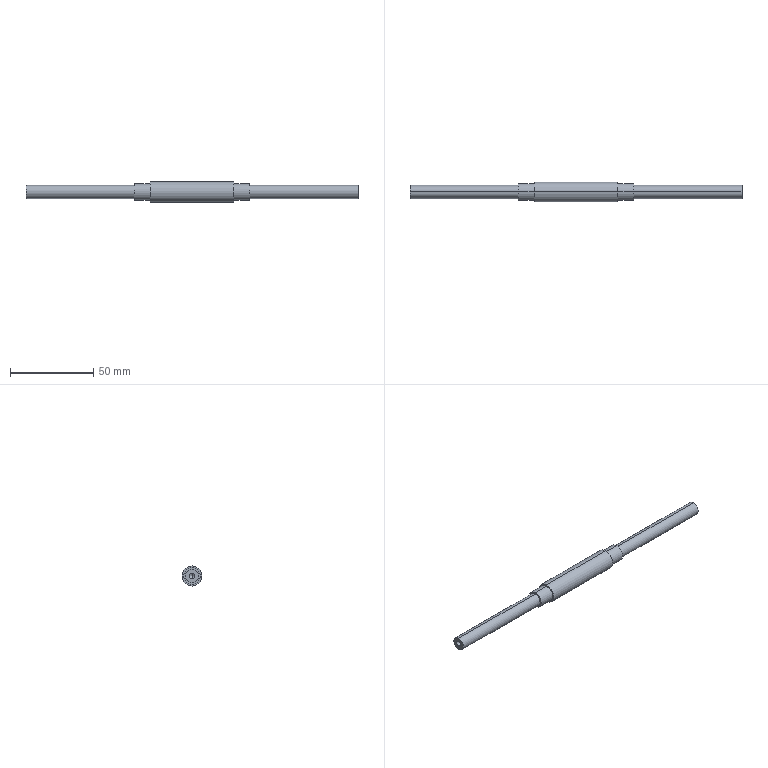Part | STEP file | MT-COMBO-119-S036 | 1 solid | 24 faces | box 199 x 12 x 12 mm | volume 13503 mm3 | cylinder 14 | plane 6 | cone 4 | commonest cylinder face diameters 3.3 x4 8 x4 10 x4 12 x2
STEP:
#1=CARTESIAN_POINT('',(89.4,0.,1.65));
#2=VERTEX_POINT('',#1);
#3=CARTESIAN_POINT('',(89.4,0.,-1.65));
#4=VERTEX_POINT('',#3);
#5=CARTESIAN_POINT('',(89.4,0.,0.));
#6=DIRECTION('',(-1.,0.,0.));
#7=DIRECTION('',(0.,0.,1.));
#8=AXIS2_PLACEMENT_3D('',#5,#6,#7);
#9=CIRCLE('',#8,1.65);
#10=EDGE_CURVE('',#2,#4,#9,.T.);
#11=ORIENTED_EDGE('',*,*,#10,.T.);
#12=CARTESIAN_POINT('',(99.5,0.,-1.65));
#13=VERTEX_POINT('',#12);
#14=CARTESIAN_POINT('',(99.5,0.,-1.65));
#15=DIRECTION('',(1.,0.,0.));
#16=VECTOR('',#15,1000.);
#17=LINE('',#14,#16);
#18=EDGE_CURVE('',#4,#13,#17,.T.);
#19=ORIENTED_EDGE('',*,*,#18,.T.);
#20=CARTESIAN_POINT('',(99.5,0.,1.65));
#21=VERTEX_POINT('',#20);
#22=CARTESIAN_POINT('',(99.5,0.,0.));
#23=DIRECTION('',(-1.,0.,0.));
#24=DIRECTION('',(0.,0.,1.));
#25=AXIS2_PLACEMENT_3D('',#22,#23,#24);
#26=CIRCLE('',#25,1.65);
#27=EDGE_CURVE('',#21,#13,#26,.T.);
#28=ORIENTED_EDGE('',*,*,#27,.F.);
#29=CARTESIAN_POINT('',(99.5,0.,1.65));
#30=DIRECTION('',(1.,0.,0.));
#31=VECTOR('',#30,1000.);
#32=LINE('',#29,#31);
#33=EDGE_CURVE('',#2,#21,#32,.T.);
#34=ORIENTED_EDGE('',*,*,#33,.F.);
#35=EDGE_LOOP('',(#11,#19,#28,#34));
#36=FACE_OUTER_BOUND('',#35,.T.);
#37=CARTESIAN_POINT('',(99.5,0.,0.));
#38=DIRECTION('',(1.,0.,0.));
#39=DIRECTION('',(0.,0.,1.));
#40=AXIS2_PLACEMENT_3D('',#37,#38,#39);
#41=CYLINDRICAL_SURFACE('',#40,1.65);
#42=ADVANCED_FACE('',(#36),#41,.F.);
#43=CARTESIAN_POINT('',(88.409,0.,0.));
#44=VERTEX_POINT('',#43);
#45=CARTESIAN_POINT('',(89.4,0.,1.65));
#46=DIRECTION('',(0.515,0.,0.8572));
#47=VECTOR('',#46,1000.);
#48=LINE('',#45,#47);
#49=EDGE_CURVE('',#44,#2,#48,.T.);
#50=ORIENTED_EDGE('',*,*,#49,.F.);
#51=CARTESIAN_POINT('',(89.4,0.,-1.65));
#52=DIRECTION('',(0.515,0.,-0.8572));
#53=VECTOR('',#52,1000.);
#54=LINE('',#51,#53);
#55=EDGE_CURVE('',#44,#4,#54,.T.);
#56=ORIENTED_EDGE('',*,*,#55,.T.);
#57=ORIENTED_EDGE('',*,*,#10,.F.);
#58=EDGE_LOOP('',(#50,#56,#57));
#59=FACE_OUTER_BOUND('',#58,.T.);
#60=CARTESIAN_POINT('',(89.4,0.,0.));
#61=DIRECTION('',(1.,0.,0.));
#62=DIRECTION('',(0.,0.,1.));
#63=AXIS2_PLACEMENT_3D('',#60,#61,#62);
#64=CONICAL_SURFACE('',#63,1.65,1.03);
#65=ADVANCED_FACE('',(#59),#64,.F.);
#66=CARTESIAN_POINT('',(-89.4,0.,-1.65));
#67=VERTEX_POINT('',#66);
#68=CARTESIAN_POINT('',(-89.4,0.,1.65));
#69=VERTEX_POINT('',#68);
#70=CARTESIAN_POINT('',(-89.4,0.,0.));
#71=DIRECTION('',(1.,0.,0.));
#72=DIRECTION('',(0.,0.,-1.));
#73=AXIS2_PLACEMENT_3D('',#70,#71,#72);
#74=CIRCLE('',#73,1.65);
#75=EDGE_CURVE('',#67,#69,#74,.T.);
#76=ORIENTED_EDGE('',*,*,#75,.T.);
#77=CARTESIAN_POINT('',(-99.5,0.,1.65));
#78=VERTEX_POINT('',#77);
#79=CARTESIAN_POINT('',(-99.5,0.,1.65));
#80=DIRECTION('',(-1.,0.,0.));
#81=VECTOR('',#80,1000.);
#82=LINE('',#79,#81);
#83=EDGE_CURVE('',#69,#78,#82,.T.);
#84=ORIENTED_EDGE('',*,*,#83,.T.);
#85=CARTESIAN_POINT('',(-99.5,0.,-1.65));
#86=VERTEX_POINT('',#85);
#87=CARTESIAN_POINT('',(-99.5,0.,0.));
#88=DIRECTION('',(1.,0.,0.));
#89=DIRECTION('',(0.,0.,-1.));
#90=AXIS2_PLACEMENT_3D('',#87,#88,#89);
#91=CIRCLE('',#90,1.65);
#92=EDGE_CURVE('',#86,#78,#91,.T.);
#93=ORIENTED_EDGE('',*,*,#92,.F.);
#94=CARTESIAN_POINT('',(-99.5,0.,-1.65));
#95=DIRECTION('',(-1.,0.,0.));
#96=VECTOR('',#95,1000.);
#97=LINE('',#94,#96);
#98=EDGE_CURVE('',#67,#86,#97,.T.);
#99=ORIENTED_EDGE('',*,*,#98,.F.);
#100=EDGE_LOOP('',(#76,#84,#93,#99));
#101=FACE_OUTER_BOUND('',#100,.T.);
#102=CARTESIAN_POINT('',(-99.5,0.,0.));
#103=DIRECTION('',(-1.,0.,0.));
#104=DIRECTION('',(0.,0.,-1.));
#105=AXIS2_PLACEMENT_3D('',#102,#103,#104);
#106=CYLINDRICAL_SURFACE('',#105,1.65);
#107=ADVANCED_FACE('',(#101),#106,.F.);
#108=CARTESIAN_POINT('',(-88.409,0.,0.));
#109=VERTEX_POINT('',#108);
#110=CARTESIAN_POINT('',(-89.4,0.,-1.65));
#111=DIRECTION('',(-0.515,0.,-0.8572));
#112=VECTOR('',#111,1000.);
#113=LINE('',#110,#112);
#114=EDGE_CURVE('',#109,#67,#113,.T.);
#115=ORIENTED_EDGE('',*,*,#114,.F.);
#116=CARTESIAN_POINT('',(-89.4,0.,1.65));
#117=DIRECTION('',(-0.515,0.,0.8572));
#118=VECTOR('',#117,1000.);
#119=LINE('',#116,#118);
#120=EDGE_CURVE('',#109,#69,#119,.T.);
#121=ORIENTED_EDGE('',*,*,#120,.T.);
#122=ORIENTED_EDGE('',*,*,#75,.F.);
#123=EDGE_LOOP('',(#115,#121,#122));
#124=FACE_OUTER_BOUND('',#123,.T.);
#125=CARTESIAN_POINT('',(-89.4,0.,0.));
#126=DIRECTION('',(-1.,0.,0.));
#127=DIRECTION('',(0.,0.,-1.));
#128=AXIS2_PLACEMENT_3D('',#125,#126,#127);
#129=CONICAL_SURFACE('',#128,1.65,1.03);
#130=ADVANCED_FACE('',(#124),#129,.F.);
#131=CARTESIAN_POINT('',(-34.5,0.,4.));
#132=VERTEX_POINT('',#131);
#133=CARTESIAN_POINT('',(-34.5,0.,-4.));
#134=VERTEX_POINT('',#133);
#135=CARTESIAN_POINT('',(-34.5,0.,0.));
#136=DIRECTION('',(1.,0.,0.));
#137=DIRECTION('',(0.,0.,-1.));
#138=AXIS2_PLACEMENT_3D('',#135,#136,#137);
#139=CIRCLE('',#138,4.);
#140=EDGE_CURVE('',#132,#134,#139,.T.);
#141=ORIENTED_EDGE('',*,*,#140,.F.);
#142=CARTESIAN_POINT('',(-99.5,0.,4.));
#143=VERTEX_POINT('',#142);
#144=CARTESIAN_POINT('',(-99.5,0.,4.));
#145=DIRECTION('',(-1.,0.,0.));
#146=VECTOR('',#145,1000.);
#147=LINE('',#144,#146);
#148=EDGE_CURVE('',#132,#143,#147,.T.);
#149=ORIENTED_EDGE('',*,*,#148,.T.);
#150=CARTESIAN_POINT('',(-99.5,0.,-4.));
#151=VERTEX_POINT('',#150);
#152=CARTESIAN_POINT('',(-99.5,0.,0.));
#153=DIRECTION('',(1.,0.,0.));
#154=DIRECTION('',(0.,0.,-1.));
#155=AXIS2_PLACEMENT_3D('',#152,#153,#154);
#156=CIRCLE('',#155,4.);
#157=EDGE_CURVE('',#143,#151,#156,.T.);
#158=ORIENTED_EDGE('',*,*,#157,.T.);
#159=CARTESIAN_POINT('',(-99.5,0.,-4.));
#160=DIRECTION('',(-1.,0.,0.));
#161=VECTOR('',#160,1000.);
#162=LINE('',#159,#161);
#163=EDGE_CURVE('',#134,#151,#162,.T.);
#164=ORIENTED_EDGE('',*,*,#163,.F.);
#165=EDGE_LOOP('',(#141,#149,#158,#164));
#166=FACE_OUTER_BOUND('',#165,.T.);
#167=CARTESIAN_POINT('',(-99.5,0.,0.));
#168=DIRECTION('',(-1.,0.,0.));
#169=DIRECTION('',(0.,0.,-1.));
#170=AXIS2_PLACEMENT_3D('',#167,#168,#169);
#171=CYLINDRICAL_SURFACE('',#170,4.);
#172=ADVANCED_FACE('',(#166),#171,.T.);
#173=CARTESIAN_POINT('',(-25.,0.,5.));
#174=VERTEX_POINT('',#173);
#175=CARTESIAN_POINT('',(-25.,0.,-5.));
#176=VERTEX_POINT('',#175);
#177=CARTESIAN_POINT('',(-25.,0.,0.));
#178=DIRECTION('',(1.,0.,0.));
#179=DIRECTION('',(0.,0.,-1.));
#180=AXIS2_PLACEMENT_3D('',#177,#178,#179);
#181=CIRCLE('',#180,5.);
#182=EDGE_CURVE('',#174,#176,#181,.T.);
#183=ORIENTED_EDGE('',*,*,#182,.F.);
#184=CARTESIAN_POINT('',(-34.5,0.,5.));
#185=VERTEX_POINT('',#184);
#186=CARTESIAN_POINT('',(-99.5,0.,5.));
#187=DIRECTION('',(-1.,0.,0.));
#188=VECTOR('',#187,1000.);
#189=LINE('',#186,#188);
#190=EDGE_CURVE('',#174,#185,#189,.T.);
#191=ORIENTED_EDGE('',*,*,#190,.T.);
#192=CARTESIAN_POINT('',(-34.5,0.,-5.));
#193=VERTEX_POINT('',#192);
#194=CARTESIAN_POINT('',(-34.5,0.,0.));
#195=DIRECTION('',(1.,0.,0.));
#196=DIRECTION('',(0.,0.,-1.));
#197=AXIS2_PLACEMENT_3D('',#194,#195,#196);
#198=CIRCLE('',#197,5.);
#199=EDGE_CURVE('',#185,#193,#198,.T.);
#200=ORIENTED_EDGE('',*,*,#199,.T.);
#201=CARTESIAN_POINT('',(-99.5,0.,-5.));
#202=DIRECTION('',(-1.,0.,0.));
#203=VECTOR('',#202,1000.);
#204=LINE('',#201,#203);
#205=EDGE_CURVE('',#176,#193,#204,.T.);
#206=ORIENTED_EDGE('',*,*,#205,.F.);
#207=EDGE_LOOP('',(#183,#191,#200,#206));
#208=FACE_OUTER_BOUND('',#207,.T.);
#209=CARTESIAN_POINT('',(-99.5,0.,0.));
#210=DIRECTION('',(-1.,0.,0.));
#211=DIRECTION('',(0.,0.,-1.));
#212=AXIS2_PLACEMENT_3D('',#209,#210,#211);
#213=CYLINDRICAL_SURFACE('',#212,5.);
#214=ADVANCED_FACE('',(#208),#213,.T.);
#215=CARTESIAN_POINT('',(25.,0.,6.));
#216=VERTEX_POINT('',#215);
#217=CARTESIAN_POINT('',(25.,0.,-6.));
#218=VERTEX_POINT('',#217);
#219=CARTESIAN_POINT('',(25.,0.,0.));
#220=DIRECTION('',(1.,0.,0.));
#221=DIRECTION('',(0.,0.,-1.));
#222=AXIS2_PLACEMENT_3D('',#219,#220,#221);
#223=CIRCLE('',#222,6.);
#224=EDGE_CURVE('',#216,#218,#223,.T.);
#225=ORIENTED_EDGE('',*,*,#224,.F.);
#226=CARTESIAN_POINT('',(-25.,0.,6.));
#227=VERTEX_POINT('',#226);
#228=CARTESIAN_POINT('',(-99.5,0.,6.));
#229=DIRECTION('',(-1.,0.,0.));
#230=VECTOR('',#229,1000.);
#231=LINE('',#228,#230);
#232=EDGE_CURVE('',#216,#227,#231,.T.);
#233=ORIENTED_EDGE('',*,*,#232,.T.);
#234=CARTESIAN_POINT('',(-25.,0.,-6.));
#235=VERTEX_POINT('',#234);
#236=CARTESIAN_POINT('',(-25.,0.,0.));
#237=DIRECTION('',(1.,0.,0.));
#238=DIRECTION('',(0.,0.,-1.));
#239=AXIS2_PLACEMENT_3D('',#236,#237,#238);
#240=CIRCLE('',#239,6.);
#241=EDGE_CURVE('',#227,#235,#240,.T.);
#242=ORIENTED_EDGE('',*,*,#241,.T.);
#243=CARTESIAN_POINT('',(-99.5,0.,-6.));
#244=DIRECTION('',(-1.,0.,0.));
#245=VECTOR('',#244,1000.);
#246=LINE('',#243,#245);
#247=EDGE_CURVE('',#218,#235,#246,.T.);
#248=ORIENTED_EDGE('',*,*,#247,.F.);
#249=EDGE_LOOP('',(#225,#233,#242,#248));
#250=FACE_OUTER_BOUND('',#249,.T.);
#251=CARTESIAN_POINT('',(-99.5,0.,0.));
#252=DIRECTION('',(-1.,0.,0.));
#253=DIRECTION('',(0.,0.,-1.));
#254=AXIS2_PLACEMENT_3D('',#251,#252,#253);
#255=CYLINDRICAL_SURFACE('',#254,6.);
#256=ADVANCED_FACE('',(#250),#255,.T.);
#257=CARTESIAN_POINT('',(34.5,0.,5.));
#258=VERTEX_POINT('',#257);
#259=CARTESIAN_POINT('',(34.5,0.,-5.));
#260=VERTEX_POINT('',#259);
#261=CARTESIAN_POINT('',(34.5,0.,0.));
#262=DIRECTION('',(1.,0.,0.));
#263=DIRECTION('',(0.,0.,-1.));
#264=AXIS2_PLACEMENT_3D('',#261,#262,#263);
#265=CIRCLE('',#264,5.);
#266=EDGE_CURVE('',#258,#260,#265,.T.);
#267=ORIENTED_EDGE('',*,*,#266,.F.);
#268=CARTESIAN_POINT('',(25.,0.,5.));
#269=VERTEX_POINT('',#268);
#270=CARTESIAN_POINT('',(-99.5,0.,5.));
#271=DIRECTION('',(-1.,0.,0.));
#272=VECTOR('',#271,1000.);
#273=LINE('',#270,#272);
#274=EDGE_CURVE('',#258,#269,#273,.T.);
#275=ORIENTED_EDGE('',*,*,#274,.T.);
#276=CARTESIAN_POINT('',(25.,0.,-5.));
#277=VERTEX_POINT('',#276);
#278=CARTESIAN_POINT('',(25.,0.,0.));
#279=DIRECTION('',(1.,0.,0.));
#280=DIRECTION('',(0.,0.,-1.));
#281=AXIS2_PLACEMENT_3D('',#278,#279,#280);
#282=CIRCLE('',#281,5.);
#283=EDGE_CURVE('',#269,#277,#282,.T.);
#284=ORIENTED_EDGE('',*,*,#283,.T.);
#285=CARTESIAN_POINT('',(-99.5,0.,-5.));
#286=DIRECTION('',(-1.,0.,0.));
#287=VECTOR('',#286,1000.);
#288=LINE('',#285,#287);
#289=EDGE_CURVE('',#260,#277,#288,.T.);
#290=ORIENTED_EDGE('',*,*,#289,.F.);
#291=EDGE_LOOP('',(#267,#275,#284,#290));
#292=FACE_OUTER_BOUND('',#291,.T.);
#293=CARTESIAN_POINT('',(-99.5,0.,0.));
#294=DIRECTION('',(-1.,0.,0.));
#295=DIRECTION('',(0.,0.,-1.));
#296=AXIS2_PLACEMENT_3D('',#293,#294,#295);
#297=CYLINDRICAL_SURFACE('',#296,5.);
#298=ADVANCED_FACE('',(#292),#297,.T.);
#299=CARTESIAN_POINT('',(99.5,0.,4.));
#300=VERTEX_POINT('',#299);
#301=CARTESIAN_POINT('',(99.5,0.,-4.));
#302=VERTEX_POINT('',#301);
#303=CARTESIAN_POINT('',(99.5,0.,0.));
#304=DIRECTION('',(1.,0.,0.));
#305=DIRECTION('',(0.,0.,-1.));
#306=AXIS2_PLACEMENT_3D('',#303,#304,#305);
#307=CIRCLE('',#306,4.);
#308=EDGE_CURVE('',#300,#302,#307,.T.);
#309=ORIENTED_EDGE('',*,*,#308,.F.);
#310=CARTESIAN_POINT('',(34.5,0.,4.));
#311=VERTEX_POINT('',#310);
#312=CARTESIAN_POINT('',(-99.5,0.,4.));
#313=DIRECTION('',(-1.,0.,0.));
#314=VECTOR('',#313,1000.);
#315=LINE('',#312,#314);
#316=EDGE_CURVE('',#300,#311,#315,.T.);
#317=ORIENTED_EDGE('',*,*,#316,.T.);
#318=CARTESIAN_POINT('',(34.5,0.,-4.));
#319=VERTEX_POINT('',#318);
#320=CARTESIAN_POINT('',(34.5,0.,0.));
#321=DIRECTION('',(1.,0.,0.));
#322=DIRECTION('',(0.,0.,-1.));
#323=AXIS2_PLACEMENT_3D('',#320,#321,#322);
#324=CIRCLE('',#323,4.);
#325=EDGE_CURVE('',#311,#319,#324,.T.);
#326=ORIENTED_EDGE('',*,*,#325,.T.);
#327=CARTESIAN_POINT('',(-99.5,0.,-4.));
#328=DIRECTION('',(-1.,0.,0.));
#329=VECTOR('',#328,1000.);
#330=LINE('',#327,#329);
#331=EDGE_CURVE('',#302,#319,#330,.T.);
#332=ORIENTED_EDGE('',*,*,#331,.F.);
#333=EDGE_LOOP('',(#309,#317,#326,#332));
#334=FACE_OUTER_BOUND('',#333,.T.);
#335=CARTESIAN_POINT('',(-99.5,0.,0.));
#336=DIRECTION('',(-1.,0.,0.));
#337=DIRECTION('',(0.,0.,-1.));
#338=AXIS2_PLACEMENT_3D('',#335,#336,#337);
#339=CYLINDRICAL_SURFACE('',#338,4.);
#340=ADVANCED_FACE('',(#334),#339,.T.);
#341=ORIENTED_EDGE('',*,*,#92,.T.);
#342=CARTESIAN_POINT('',(-99.5,0.,0.));
#343=DIRECTION('',(1.,0.,0.));
#344=DIRECTION('',(0.,0.,-1.));
#345=AXIS2_PLACEMENT_3D('',#342,#343,#344);
#346=CIRCLE('',#345,1.65);
#347=EDGE_CURVE('',#78,#86,#346,.T.);
#348=ORIENTED_EDGE('',*,*,#347,.T.);
#349=EDGE_LOOP('',(#341,#348));
#350=FACE_BOUND('',#349,.T.);
#351=CARTESIAN_POINT('',(-99.5,0.,0.));
#352=DIRECTION('',(1.,0.,0.));
#353=DIRECTION('',(0.,0.,-1.));
#354=AXIS2_PLACEMENT_3D('',#351,#352,#353);
#355=CIRCLE('',#354,4.);
#356=EDGE_CURVE('',#151,#143,#355,.T.);
#357=ORIENTED_EDGE('',*,*,#356,.F.);
#358=ORIENTED_EDGE('',*,*,#157,.F.);
#359=EDGE_LOOP('',(#357,#358));
#360=FACE_OUTER_BOUND('',#359,.T.);
#361=CARTESIAN_POINT('',(-99.5,0.,0.));
#362=DIRECTION('',(1.,0.,0.));
#363=DIRECTION('',(0.,0.,1.));
#364=AXIS2_PLACEMENT_3D('',#361,#362,#363);
#365=PLANE('',#364);
#366=ADVANCED_FACE('',(#350,#360),#365,.F.);
#367=ORIENTED_EDGE('',*,*,#27,.T.);
#368=CARTESIAN_POINT('',(99.5,0.,0.));
#369=DIRECTION('',(-1.,0.,0.));
#370=DIRECTION('',(0.,0.,1.));
#371=AXIS2_PLACEMENT_3D('',#368,#369,#370);
#372=CIRCLE('',#371,1.65);
#373=EDGE_CURVE('',#13,#21,#372,.T.);
#374=ORIENTED_EDGE('',*,*,#373,.T.);
#375=EDGE_LOOP('',(#367,#374));
#376=FACE_BOUND('',#375,.T.);
#377=CARTESIAN_POINT('',(99.5,0.,0.));
#378=DIRECTION('',(1.,0.,0.));
#379=DIRECTION('',(0.,0.,-1.));
#380=AXIS2_PLACEMENT_3D('',#377,#378,#379);
#381=CIRCLE('',#380,4.);
#382=EDGE_CURVE('',#302,#300,#381,.T.);
#383=ORIENTED_EDGE('',*,*,#382,.T.);
#384=ORIENTED_EDGE('',*,*,#308,.T.);
#385=EDGE_LOOP('',(#383,#384));
#386=FACE_OUTER_BOUND('',#385,.T.);
#387=CARTESIAN_POINT('',(99.5,0.,0.));
#388=DIRECTION('',(-1.,0.,0.));
#389=DIRECTION('',(0.,0.,-1.));
#390=AXIS2_PLACEMENT_3D('',#387,#388,#389);
#391=PLANE('',#390);
#392=ADVANCED_FACE('',(#376,#386),#391,.F.);
#393=ORIENTED_EDGE('',*,*,#316,.F.);
#394=ORIENTED_EDGE('',*,*,#382,.F.);
#395=ORIENTED_EDGE('',*,*,#331,.T.);
#396=CARTESIAN_POINT('',(34.5,0.,0.));
#397=DIRECTION('',(1.,0.,0.));
#398=DIRECTION('',(0.,0.,-1.));
#399=AXIS2_PLACEMENT_3D('',#396,#397,#398);
#400=CIRCLE('',#399,4.);
#401=EDGE_CURVE('',#319,#311,#400,.T.);
#402=ORIENTED_EDGE('',*,*,#401,.T.);
#403=EDGE_LOOP('',(#393,#394,#395,#402));
#404=FACE_OUTER_BOUND('',#403,.T.);
#405=CARTESIAN_POINT('',(-99.5,0.,0.));
#406=DIRECTION('',(-1.,0.,0.));
#407=DIRECTION('',(0.,0.,-1.));
#408=AXIS2_PLACEMENT_3D('',#405,#406,#407);
#409=CYLINDRICAL_SURFACE('',#408,4.);
#410=ADVANCED_FACE('',(#404),#409,.T.);
#411=CARTESIAN_POINT('',(34.5,0.,0.));
#412=DIRECTION('',(1.,0.,0.));
#413=DIRECTION('',(0.,0.,-1.));
#414=AXIS2_PLACEMENT_3D('',#411,#412,#413);
#415=CIRCLE('',#414,5.);
#416=EDGE_CURVE('',#260,#258,#415,.T.);
#417=ORIENTED_EDGE('',*,*,#416,.T.);
#418=ORIENTED_EDGE('',*,*,#266,.T.);
#419=EDGE_LOOP('',(#417,#418));
#420=FACE_OUTER_BOUND('',#419,.T.);
#421=ORIENTED_EDGE('',*,*,#401,.F.);
#422=ORIENTED_EDGE('',*,*,#325,.F.);
#423=EDGE_LOOP('',(#421,#422));
#424=FACE_BOUND('',#423,.T.);
#425=CARTESIAN_POINT('',(34.5,5.,0.));
#426=DIRECTION('',(-1.,0.,0.));
#427=DIRECTION('',(0.,0.,-1.));
#428=AXIS2_PLACEMENT_3D('',#425,#426,#427);
#429=PLANE('',#428);
#430=ADVANCED_FACE('',(#420,#424),#429,.F.);
#431=ORIENTED_EDGE('',*,*,#274,.F.);
#432=ORIENTED_EDGE('',*,*,#416,.F.);
#433=ORIENTED_EDGE('',*,*,#289,.T.);
#434=CARTESIAN_POINT('',(25.,0.,0.));
#435=DIRECTION('',(1.,0.,0.));
#436=DIRECTION('',(0.,0.,-1.));
#437=AXIS2_PLACEMENT_3D('',#434,#435,#436);
#438=CIRCLE('',#437,5.);
#439=EDGE_CURVE('',#277,#269,#438,.T.);
#440=ORIENTED_EDGE('',*,*,#439,.T.);
#441=EDGE_LOOP('',(#431,#432,#433,#440));
#442=FACE_OUTER_BOUND('',#441,.T.);
#443=CARTESIAN_POINT('',(-99.5,0.,0.));
#444=DIRECTION('',(-1.,0.,0.));
#445=DIRECTION('',(0.,0.,-1.));
#446=AXIS2_PLACEMENT_3D('',#443,#444,#445);
#447=CYLINDRICAL_SURFACE('',#446,5.);
#448=ADVANCED_FACE('',(#442),#447,.T.);
#449=CARTESIAN_POINT('',(25.,0.,0.));
#450=DIRECTION('',(1.,0.,0.));
#451=DIRECTION('',(0.,0.,-1.));
#452=AXIS2_PLACEMENT_3D('',#449,#450,#451);
#453=CIRCLE('',#452,6.);
#454=EDGE_CURVE('',#218,#216,#453,.T.);
#455=ORIENTED_EDGE('',*,*,#454,.T.);
#456=ORIENTED_EDGE('',*,*,#224,.T.);
#457=EDGE_LOOP('',(#455,#456));
#458=FACE_OUTER_BOUND('',#457,.T.);
#459=ORIENTED_EDGE('',*,*,#439,.F.);
#460=ORIENTED_EDGE('',*,*,#283,.F.);
#461=EDGE_LOOP('',(#459,#460));
#462=FACE_BOUND('',#461,.T.);
#463=CARTESIAN_POINT('',(25.,6.,0.));
#464=DIRECTION('',(-1.,0.,0.));
#465=DIRECTION('',(0.,0.,-1.));
#466=AXIS2_PLACEMENT_3D('',#463,#464,#465);
#467=PLANE('',#466);
#468=ADVANCED_FACE('',(#458,#462),#467,.F.);
#469=ORIENTED_EDGE('',*,*,#232,.F.);
#470=ORIENTED_EDGE('',*,*,#454,.F.);
#471=ORIENTED_EDGE('',*,*,#247,.T.);
#472=CARTESIAN_POINT('',(-25.,0.,0.));
#473=DIRECTION('',(1.,0.,0.));
#474=DIRECTION('',(0.,0.,-1.));
#475=AXIS2_PLACEMENT_3D('',#472,#473,#474);
#476=CIRCLE('',#475,6.);
#477=EDGE_CURVE('',#235,#227,#476,.T.);
#478=ORIENTED_EDGE('',*,*,#477,.T.);
#479=EDGE_LOOP('',(#469,#470,#471,#478));
#480=FACE_OUTER_BOUND('',#479,.T.);
#481=CARTESIAN_POINT('',(-99.5,0.,0.));
#482=DIRECTION('',(-1.,0.,0.));
#483=DIRECTION('',(0.,0.,-1.));
#484=AXIS2_PLACEMENT_3D('',#481,#482,#483);
#485=CYLINDRICAL_SURFACE('',#484,6.);
#486=ADVANCED_FACE('',(#480),#485,.T.);
#487=CARTESIAN_POINT('',(-25.,0.,0.));
#488=DIRECTION('',(1.,0.,0.));
#489=DIRECTION('',(0.,0.,-1.));
#490=AXIS2_PLACEMENT_3D('',#487,#488,#489);
#491=CIRCLE('',#490,5.);
#492=EDGE_CURVE('',#176,#174,#491,.T.);
#493=ORIENTED_EDGE('',*,*,#492,.T.);
#494=ORIENTED_EDGE('',*,*,#182,.T.);
#495=EDGE_LOOP('',(#493,#494));
#496=FACE_BOUND('',#495,.T.);
#497=ORIENTED_EDGE('',*,*,#477,.F.);
#498=ORIENTED_EDGE('',*,*,#241,.F.);
#499=EDGE_LOOP('',(#497,#498));
#500=FACE_OUTER_BOUND('',#499,.T.);
#501=CARTESIAN_POINT('',(-25.,6.,0.));
#502=DIRECTION('',(1.,0.,0.));
#503=DIRECTION('',(0.,0.,1.));
#504=AXIS2_PLACEMENT_3D('',#501,#502,#503);
#505=PLANE('',#504);
#506=ADVANCED_FACE('',(#496,#500),#505,.F.);
#507=ORIENTED_EDGE('',*,*,#190,.F.);
#508=ORIENTED_EDGE('',*,*,#492,.F.);
#509=ORIENTED_EDGE('',*,*,#205,.T.);
#510=CARTESIAN_POINT('',(-34.5,0.,0.));
#511=DIRECTION('',(1.,0.,0.));
#512=DIRECTION('',(0.,0.,-1.));
#513=AXIS2_PLACEMENT_3D('',#510,#511,#512);
#514=CIRCLE('',#513,5.);
#515=EDGE_CURVE('',#193,#185,#514,.T.);
#516=ORIENTED_EDGE('',*,*,#515,.T.);
#517=EDGE_LOOP('',(#507,#508,#509,#516));
#518=FACE_OUTER_BOUND('',#517,.T.);
#519=CARTESIAN_POINT('',(-99.5,0.,0.));
#520=DIRECTION('',(-1.,0.,0.));
#521=DIRECTION('',(0.,0.,-1.));
#522=AXIS2_PLACEMENT_3D('',#519,#520,#521);
#523=CYLINDRICAL_SURFACE('',#522,5.);
#524=ADVANCED_FACE('',(#518),#523,.T.);
#525=CARTESIAN_POINT('',(-34.5,0.,0.));
#526=DIRECTION('',(1.,0.,0.));
#527=DIRECTION('',(0.,0.,-1.));
#528=AXIS2_PLACEMENT_3D('',#525,#526,#527);
#529=CIRCLE('',#528,4.);
#530=EDGE_CURVE('',#134,#132,#529,.T.);
#531=ORIENTED_EDGE('',*,*,#530,.T.);
#532=ORIENTED_EDGE('',*,*,#140,.T.);
#533=EDGE_LOOP('',(#531,#532));
#534=FACE_BOUND('',#533,.T.);
#535=ORIENTED_EDGE('',*,*,#515,.F.);
#536=ORIENTED_EDGE('',*,*,#199,.F.);
#537=EDGE_LOOP('',(#535,#536));
#538=FACE_OUTER_BOUND('',#537,.T.);
#539=CARTESIAN_POINT('',(-34.5,5.,0.));
#540=DIRECTION('',(1.,0.,0.));
#541=DIRECTION('',(0.,0.,1.));
#542=AXIS2_PLACEMENT_3D('',#539,#540,#541);
#543=PLANE('',#542);
#544=ADVANCED_FACE('',(#534,#538),#543,.F.);
#545=ORIENTED_EDGE('',*,*,#148,.F.);
#546=ORIENTED_EDGE('',*,*,#530,.F.);
#547=ORIENTED_EDGE('',*,*,#163,.T.);
#548=ORIENTED_EDGE('',*,*,#356,.T.);
#549=EDGE_LOOP('',(#545,#546,#547,#548));
#550=FACE_OUTER_BOUND('',#549,.T.);
#551=CARTESIAN_POINT('',(-99.5,0.,0.));
#552=DIRECTION('',(-1.,0.,0.));
#553=DIRECTION('',(0.,0.,-1.));
#554=AXIS2_PLACEMENT_3D('',#551,#552,#553);
#555=CYLINDRICAL_SURFACE('',#554,4.);
#556=ADVANCED_FACE('',(#550),#555,.T.);
#557=ORIENTED_EDGE('',*,*,#120,.F.);
#558=ORIENTED_EDGE('',*,*,#114,.T.);
#559=CARTESIAN_POINT('',(-89.4,0.,0.));
#560=DIRECTION('',(1.,0.,0.));
#561=DIRECTION('',(0.,0.,-1.));
#562=AXIS2_PLACEMENT_3D('',#559,#560,#561);
#563=CIRCLE('',#562,1.65);
#564=EDGE_CURVE('',#69,#67,#563,.T.);
#565=ORIENTED_EDGE('',*,*,#564,.F.);
#566=EDGE_LOOP('',(#557,#558,#565));
#567=FACE_OUTER_BOUND('',#566,.T.);
#568=CARTESIAN_POINT('',(-89.4,0.,0.));
#569=DIRECTION('',(-1.,0.,0.));
#570=DIRECTION('',(0.,0.,-1.));
#571=AXIS2_PLACEMENT_3D('',#568,#569,#570);
#572=CONICAL_SURFACE('',#571,1.65,1.03);
#573=ADVANCED_FACE('',(#567),#572,.F.);
#574=ORIENTED_EDGE('',*,*,#83,.F.);
#575=ORIENTED_EDGE('',*,*,#564,.T.);
#576=ORIENTED_EDGE('',*,*,#98,.T.);
#577=ORIENTED_EDGE('',*,*,#347,.F.);
#578=EDGE_LOOP('',(#574,#575,#576,#577));
#579=FACE_OUTER_BOUND('',#578,.T.);
#580=CARTESIAN_POINT('',(-99.5,0.,0.));
#581=DIRECTION('',(-1.,0.,0.));
#582=DIRECTION('',(0.,0.,-1.));
#583=AXIS2_PLACEMENT_3D('',#580,#581,#582);
#584=CYLINDRICAL_SURFACE('',#583,1.65);
#585=ADVANCED_FACE('',(#579),#584,.F.);
#586=ORIENTED_EDGE('',*,*,#55,.F.);
#587=ORIENTED_EDGE('',*,*,#49,.T.);
#588=CARTESIAN_POINT('',(89.4,0.,0.));
#589=DIRECTION('',(-1.,0.,0.));
#590=DIRECTION('',(0.,0.,1.));
#591=AXIS2_PLACEMENT_3D('',#588,#589,#590);
#592=CIRCLE('',#591,1.65);
#593=EDGE_CURVE('',#4,#2,#592,.T.);
#594=ORIENTED_EDGE('',*,*,#593,.F.);
#595=EDGE_LOOP('',(#586,#587,#594));
#596=FACE_OUTER_BOUND('',#595,.T.);
#597=CARTESIAN_POINT('',(89.4,0.,0.));
#598=DIRECTION('',(1.,0.,0.));
#599=DIRECTION('',(0.,0.,1.));
#600=AXIS2_PLACEMENT_3D('',#597,#598,#599);
#601=CONICAL_SURFACE('',#600,1.65,1.03);
#602=ADVANCED_FACE('',(#596),#601,.F.);
#603=ORIENTED_EDGE('',*,*,#18,.F.);
#604=ORIENTED_EDGE('',*,*,#593,.T.);
#605=ORIENTED_EDGE('',*,*,#33,.T.);
#606=ORIENTED_EDGE('',*,*,#373,.F.);
#607=EDGE_LOOP('',(#603,#604,#605,#606));
#608=FACE_OUTER_BOUND('',#607,.T.);
#609=CARTESIAN_POINT('',(99.5,0.,0.));
#610=DIRECTION('',(1.,0.,0.));
#611=DIRECTION('',(0.,0.,1.));
#612=AXIS2_PLACEMENT_3D('',#609,#610,#611);
#613=CYLINDRICAL_SURFACE('',#612,1.65);
#614=ADVANCED_FACE('',(#608),#613,.F.);
#615=CLOSED_SHELL('',(#42,#65,#107,#130,#172,#214,#256,#298,#340,#366,#392,#410,#430,#448,#468,#486,#506,#524,#544,#556,#573,#585,#602,#614));
#616=MANIFOLD_SOLID_BREP('',#615);
#617=CARTESIAN_POINT('',(0.,0.,0.));
#618=DIRECTION('',(0.,0.,1.));
#619=DIRECTION('',(1.,0.,0.));
#620=AXIS2_PLACEMENT_3D('',#617,#618,#619);
#621=(LENGTH_UNIT()NAMED_UNIT(*)SI_UNIT(.MILLI.,.METRE.));
#622=UNCERTAINTY_MEASURE_WITH_UNIT(LENGTH_MEASURE(0.00001),#621,'','');
#623=(NAMED_UNIT(*)PLANE_ANGLE_UNIT()SI_UNIT($,.RADIAN.));
#624=(NAMED_UNIT(*)SI_UNIT($,.STERADIAN.)SOLID_ANGLE_UNIT());
#625=(GEOMETRIC_REPRESENTATION_CONTEXT(3)GLOBAL_UNCERTAINTY_ASSIGNED_CONTEXT((#622))GLOBAL_UNIT_ASSIGNED_CONTEXT((#621,#623,#624))REPRESENTATION_CONTEXT('',''));
#626=ADVANCED_BREP_SHAPE_REPRESENTATION('',(#616,#620),#625);